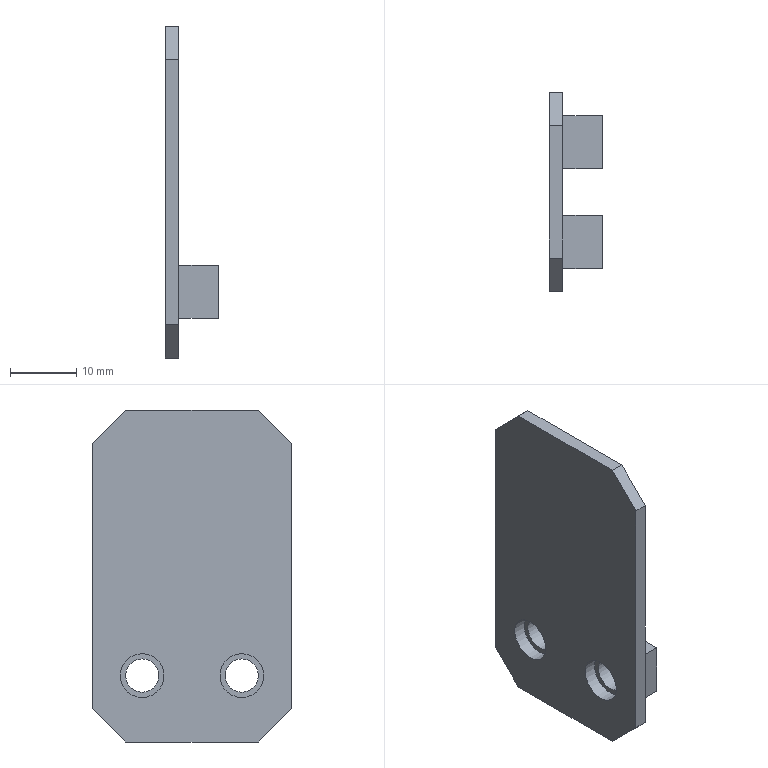Part | NX | features 5003_223_Plate 2 | 1 solid | 26 faces | box 8 x 30 x 50 mm | volume 3296 mm3 | plane 22 | cylinder 4 | commonest cylinder face diameters 5 x2 6.6 x2
STEP:
#1=CARTESIAN_POINT('',(193.825,63.4,-12.));
#2=VERTEX_POINT('',#1);
#3=CARTESIAN_POINT('',(193.825,68.4,-7.));
#4=VERTEX_POINT('',#3);
#5=CARTESIAN_POINT('',(193.825,63.4,-12.));
#6=DIRECTION('',(0.,0.7071,0.7071));
#7=VECTOR('',#6,1000.);
#8=LINE('',#5,#7);
#9=EDGE_CURVE('',#2,#4,#8,.T.);
#10=ORIENTED_EDGE('',*,*,#9,.T.);
#11=CARTESIAN_POINT('',(193.825,88.4,-7.));
#12=VERTEX_POINT('',#11);
#13=CARTESIAN_POINT('',(193.825,88.4,-7.));
#14=DIRECTION('',(0.,1.,0.));
#15=VECTOR('',#14,1000.);
#16=LINE('',#13,#15);
#17=EDGE_CURVE('',#4,#12,#16,.T.);
#18=ORIENTED_EDGE('',*,*,#17,.T.);
#19=CARTESIAN_POINT('',(193.825,93.4,-12.));
#20=VERTEX_POINT('',#19);
#21=CARTESIAN_POINT('',(193.825,93.4,-12.));
#22=DIRECTION('',(0.,0.7071,-0.7071));
#23=VECTOR('',#22,1000.);
#24=LINE('',#21,#23);
#25=EDGE_CURVE('',#12,#20,#24,.T.);
#26=ORIENTED_EDGE('',*,*,#25,.T.);
#27=CARTESIAN_POINT('',(193.825,93.4,-52.));
#28=VERTEX_POINT('',#27);
#29=CARTESIAN_POINT('',(193.825,93.4,-52.));
#30=DIRECTION('',(0.,0.,-1.));
#31=VECTOR('',#30,1000.);
#32=LINE('',#29,#31);
#33=EDGE_CURVE('',#20,#28,#32,.T.);
#34=ORIENTED_EDGE('',*,*,#33,.T.);
#35=CARTESIAN_POINT('',(193.825,88.4,-57.));
#36=VERTEX_POINT('',#35);
#37=CARTESIAN_POINT('',(193.825,88.4,-57.));
#38=DIRECTION('',(0.,-0.7071,-0.7071));
#39=VECTOR('',#38,1000.);
#40=LINE('',#37,#39);
#41=EDGE_CURVE('',#28,#36,#40,.T.);
#42=ORIENTED_EDGE('',*,*,#41,.T.);
#43=CARTESIAN_POINT('',(193.825,68.4,-57.));
#44=VERTEX_POINT('',#43);
#45=CARTESIAN_POINT('',(193.825,88.4,-57.));
#46=DIRECTION('',(0.,-1.,0.));
#47=VECTOR('',#46,1000.);
#48=LINE('',#45,#47);
#49=EDGE_CURVE('',#36,#44,#48,.T.);
#50=ORIENTED_EDGE('',*,*,#49,.T.);
#51=CARTESIAN_POINT('',(193.825,63.4,-52.));
#52=VERTEX_POINT('',#51);
#53=CARTESIAN_POINT('',(193.825,68.4,-57.));
#54=DIRECTION('',(0.,-0.7071,0.7071));
#55=VECTOR('',#54,1000.);
#56=LINE('',#53,#55);
#57=EDGE_CURVE('',#44,#52,#56,.T.);
#58=ORIENTED_EDGE('',*,*,#57,.T.);
#59=CARTESIAN_POINT('',(193.825,63.4,-52.));
#60=DIRECTION('',(0.,0.,1.));
#61=VECTOR('',#60,1000.);
#62=LINE('',#59,#61);
#63=EDGE_CURVE('',#52,#2,#62,.T.);
#64=ORIENTED_EDGE('',*,*,#63,.T.);
#65=EDGE_LOOP('',(#10,#18,#26,#34,#42,#50,#58,#64));
#66=FACE_BOUND('',#65,.T.);
#67=CARTESIAN_POINT('',(193.825,85.9,-50.3));
#68=VERTEX_POINT('',#67);
#69=CARTESIAN_POINT('',(193.825,85.9,-47.));
#70=DIRECTION('',(-1.,0.,0.));
#71=DIRECTION('',(0.,0.,-1.));
#72=AXIS2_PLACEMENT_3D('',#69,#70,#71);
#73=CIRCLE('',#72,3.3);
#74=EDGE_CURVE('',#68,#68,#73,.T.);
#75=ORIENTED_EDGE('',*,*,#74,.F.);
#76=EDGE_LOOP('',(#75));
#77=FACE_BOUND('',#76,.T.);
#78=CARTESIAN_POINT('',(193.825,70.9,-50.3));
#79=VERTEX_POINT('',#78);
#80=CARTESIAN_POINT('',(193.825,70.9,-47.));
#81=DIRECTION('',(-1.,0.,0.));
#82=DIRECTION('',(0.,0.,-1.));
#83=AXIS2_PLACEMENT_3D('',#80,#81,#82);
#84=CIRCLE('',#83,3.3);
#85=EDGE_CURVE('',#79,#79,#84,.T.);
#86=ORIENTED_EDGE('',*,*,#85,.F.);
#87=EDGE_LOOP('',(#86));
#88=FACE_BOUND('',#87,.T.);
#89=CARTESIAN_POINT('',(193.825,93.4,-57.));
#90=DIRECTION('',(1.,0.,0.));
#91=DIRECTION('',(0.,0.,1.));
#92=AXIS2_PLACEMENT_3D('',#89,#90,#91);
#93=PLANE('',#92);
#94=ADVANCED_FACE('',(#66,#77,#88),#93,.F.);
#95=CARTESIAN_POINT('',(195.825,89.9,-51.));
#96=VERTEX_POINT('',#95);
#97=CARTESIAN_POINT('',(195.825,81.9,-51.));
#98=VERTEX_POINT('',#97);
#99=CARTESIAN_POINT('',(195.825,81.9,-51.));
#100=DIRECTION('',(0.,-1.,0.));
#101=VECTOR('',#100,1000.);
#102=LINE('',#99,#101);
#103=EDGE_CURVE('',#96,#98,#102,.T.);
#104=ORIENTED_EDGE('',*,*,#103,.T.);
#105=CARTESIAN_POINT('',(195.825,81.9,-43.));
#106=VERTEX_POINT('',#105);
#107=CARTESIAN_POINT('',(195.825,81.9,-43.));
#108=DIRECTION('',(0.,0.,1.));
#109=VECTOR('',#108,1000.);
#110=LINE('',#107,#109);
#111=EDGE_CURVE('',#98,#106,#110,.T.);
#112=ORIENTED_EDGE('',*,*,#111,.T.);
#113=CARTESIAN_POINT('',(195.825,89.9,-43.));
#114=VERTEX_POINT('',#113);
#115=CARTESIAN_POINT('',(195.825,81.9,-43.));
#116=DIRECTION('',(0.,1.,0.));
#117=VECTOR('',#116,1000.);
#118=LINE('',#115,#117);
#119=EDGE_CURVE('',#106,#114,#118,.T.);
#120=ORIENTED_EDGE('',*,*,#119,.T.);
#121=CARTESIAN_POINT('',(195.825,89.9,-43.));
#122=DIRECTION('',(0.,0.,-1.));
#123=VECTOR('',#122,1000.);
#124=LINE('',#121,#123);
#125=EDGE_CURVE('',#114,#96,#124,.T.);
#126=ORIENTED_EDGE('',*,*,#125,.T.);
#127=EDGE_LOOP('',(#104,#112,#120,#126));
#128=FACE_BOUND('',#127,.T.);
#129=CARTESIAN_POINT('',(195.825,74.9,-51.));
#130=VERTEX_POINT('',#129);
#131=CARTESIAN_POINT('',(195.825,66.9,-51.));
#132=VERTEX_POINT('',#131);
#133=CARTESIAN_POINT('',(195.825,66.9,-51.));
#134=DIRECTION('',(0.,-1.,0.));
#135=VECTOR('',#134,1000.);
#136=LINE('',#133,#135);
#137=EDGE_CURVE('',#130,#132,#136,.T.);
#138=ORIENTED_EDGE('',*,*,#137,.T.);
#139=CARTESIAN_POINT('',(195.825,66.9,-43.));
#140=VERTEX_POINT('',#139);
#141=CARTESIAN_POINT('',(195.825,66.9,-43.));
#142=DIRECTION('',(0.,0.,1.));
#143=VECTOR('',#142,1000.);
#144=LINE('',#141,#143);
#145=EDGE_CURVE('',#132,#140,#144,.T.);
#146=ORIENTED_EDGE('',*,*,#145,.T.);
#147=CARTESIAN_POINT('',(195.825,74.9,-43.));
#148=VERTEX_POINT('',#147);
#149=CARTESIAN_POINT('',(195.825,66.9,-43.));
#150=DIRECTION('',(0.,1.,0.));
#151=VECTOR('',#150,1000.);
#152=LINE('',#149,#151);
#153=EDGE_CURVE('',#140,#148,#152,.T.);
#154=ORIENTED_EDGE('',*,*,#153,.T.);
#155=CARTESIAN_POINT('',(195.825,74.9,-43.));
#156=DIRECTION('',(0.,0.,-1.));
#157=VECTOR('',#156,1000.);
#158=LINE('',#155,#157);
#159=EDGE_CURVE('',#148,#130,#158,.T.);
#160=ORIENTED_EDGE('',*,*,#159,.T.);
#161=EDGE_LOOP('',(#138,#146,#154,#160));
#162=FACE_BOUND('',#161,.T.);
#163=CARTESIAN_POINT('',(195.825,63.4,-12.));
#164=VERTEX_POINT('',#163);
#165=CARTESIAN_POINT('',(195.825,68.4,-7.));
#166=VERTEX_POINT('',#165);
#167=CARTESIAN_POINT('',(195.825,63.4,-12.));
#168=DIRECTION('',(0.,0.7071,0.7071));
#169=VECTOR('',#168,1000.);
#170=LINE('',#167,#169);
#171=EDGE_CURVE('',#164,#166,#170,.T.);
#172=ORIENTED_EDGE('',*,*,#171,.F.);
#173=CARTESIAN_POINT('',(195.825,63.4,-52.));
#174=VERTEX_POINT('',#173);
#175=CARTESIAN_POINT('',(195.825,63.4,-52.));
#176=DIRECTION('',(0.,0.,1.));
#177=VECTOR('',#176,1000.);
#178=LINE('',#175,#177);
#179=EDGE_CURVE('',#174,#164,#178,.T.);
#180=ORIENTED_EDGE('',*,*,#179,.F.);
#181=CARTESIAN_POINT('',(195.825,68.4,-57.));
#182=VERTEX_POINT('',#181);
#183=CARTESIAN_POINT('',(195.825,68.4,-57.));
#184=DIRECTION('',(0.,-0.7071,0.7071));
#185=VECTOR('',#184,1000.);
#186=LINE('',#183,#185);
#187=EDGE_CURVE('',#182,#174,#186,.T.);
#188=ORIENTED_EDGE('',*,*,#187,.F.);
#189=CARTESIAN_POINT('',(195.825,88.4,-57.));
#190=VERTEX_POINT('',#189);
#191=CARTESIAN_POINT('',(195.825,88.4,-57.));
#192=DIRECTION('',(0.,-1.,0.));
#193=VECTOR('',#192,1000.);
#194=LINE('',#191,#193);
#195=EDGE_CURVE('',#190,#182,#194,.T.);
#196=ORIENTED_EDGE('',*,*,#195,.F.);
#197=CARTESIAN_POINT('',(195.825,93.4,-52.));
#198=VERTEX_POINT('',#197);
#199=CARTESIAN_POINT('',(195.825,88.4,-57.));
#200=DIRECTION('',(0.,-0.7071,-0.7071));
#201=VECTOR('',#200,1000.);
#202=LINE('',#199,#201);
#203=EDGE_CURVE('',#198,#190,#202,.T.);
#204=ORIENTED_EDGE('',*,*,#203,.F.);
#205=CARTESIAN_POINT('',(195.825,93.4,-12.));
#206=VERTEX_POINT('',#205);
#207=CARTESIAN_POINT('',(195.825,93.4,-52.));
#208=DIRECTION('',(0.,0.,-1.));
#209=VECTOR('',#208,1000.);
#210=LINE('',#207,#209);
#211=EDGE_CURVE('',#206,#198,#210,.T.);
#212=ORIENTED_EDGE('',*,*,#211,.F.);
#213=CARTESIAN_POINT('',(195.825,88.4,-7.));
#214=VERTEX_POINT('',#213);
#215=CARTESIAN_POINT('',(195.825,93.4,-12.));
#216=DIRECTION('',(0.,0.7071,-0.7071));
#217=VECTOR('',#216,1000.);
#218=LINE('',#215,#217);
#219=EDGE_CURVE('',#214,#206,#218,.T.);
#220=ORIENTED_EDGE('',*,*,#219,.F.);
#221=CARTESIAN_POINT('',(195.825,88.4,-7.));
#222=DIRECTION('',(0.,1.,0.));
#223=VECTOR('',#222,1000.);
#224=LINE('',#221,#223);
#225=EDGE_CURVE('',#166,#214,#224,.T.);
#226=ORIENTED_EDGE('',*,*,#225,.F.);
#227=EDGE_LOOP('',(#172,#180,#188,#196,#204,#212,#220,#226));
#228=FACE_BOUND('',#227,.T.);
#229=CARTESIAN_POINT('',(195.825,93.4,-57.));
#230=DIRECTION('',(1.,0.,0.));
#231=DIRECTION('',(0.,0.,1.));
#232=AXIS2_PLACEMENT_3D('',#229,#230,#231);
#233=PLANE('',#232);
#234=ADVANCED_FACE('',(#128,#162,#228),#233,.T.);
#235=ORIENTED_EDGE('',*,*,#171,.T.);
#236=CARTESIAN_POINT('',(193.825,68.4,-7.));
#237=DIRECTION('',(1.,0.,0.));
#238=VECTOR('',#237,1000.);
#239=LINE('',#236,#238);
#240=EDGE_CURVE('',#4,#166,#239,.T.);
#241=ORIENTED_EDGE('',*,*,#240,.F.);
#242=ORIENTED_EDGE('',*,*,#9,.F.);
#243=CARTESIAN_POINT('',(193.825,63.4,-12.));
#244=DIRECTION('',(1.,0.,0.));
#245=VECTOR('',#244,1000.);
#246=LINE('',#243,#245);
#247=EDGE_CURVE('',#2,#164,#246,.T.);
#248=ORIENTED_EDGE('',*,*,#247,.T.);
#249=EDGE_LOOP('',(#235,#241,#242,#248));
#250=FACE_BOUND('',#249,.T.);
#251=CARTESIAN_POINT('',(193.825,63.4,-12.));
#252=DIRECTION('',(0.,0.7071,-0.7071));
#253=DIRECTION('',(0.,-0.7071,-0.7071));
#254=AXIS2_PLACEMENT_3D('',#251,#252,#253);
#255=PLANE('',#254);
#256=ADVANCED_FACE('',(#250),#255,.F.);
#257=ORIENTED_EDGE('',*,*,#225,.T.);
#258=CARTESIAN_POINT('',(193.825,88.4,-7.));
#259=DIRECTION('',(1.,0.,0.));
#260=VECTOR('',#259,1000.);
#261=LINE('',#258,#260);
#262=EDGE_CURVE('',#12,#214,#261,.T.);
#263=ORIENTED_EDGE('',*,*,#262,.F.);
#264=ORIENTED_EDGE('',*,*,#17,.F.);
#265=ORIENTED_EDGE('',*,*,#240,.T.);
#266=EDGE_LOOP('',(#257,#263,#264,#265));
#267=FACE_BOUND('',#266,.T.);
#268=CARTESIAN_POINT('',(193.825,88.4,-7.));
#269=DIRECTION('',(0.,0.,-1.));
#270=DIRECTION('',(1.,0.,0.));
#271=AXIS2_PLACEMENT_3D('',#268,#269,#270);
#272=PLANE('',#271);
#273=ADVANCED_FACE('',(#267),#272,.F.);
#274=ORIENTED_EDGE('',*,*,#219,.T.);
#275=CARTESIAN_POINT('',(193.825,93.4,-12.));
#276=DIRECTION('',(1.,0.,0.));
#277=VECTOR('',#276,1000.);
#278=LINE('',#275,#277);
#279=EDGE_CURVE('',#20,#206,#278,.T.);
#280=ORIENTED_EDGE('',*,*,#279,.F.);
#281=ORIENTED_EDGE('',*,*,#25,.F.);
#282=ORIENTED_EDGE('',*,*,#262,.T.);
#283=EDGE_LOOP('',(#274,#280,#281,#282));
#284=FACE_BOUND('',#283,.T.);
#285=CARTESIAN_POINT('',(193.825,93.4,-12.));
#286=DIRECTION('',(0.,-0.7071,-0.7071));
#287=DIRECTION('',(0.,-0.7071,0.7071));
#288=AXIS2_PLACEMENT_3D('',#285,#286,#287);
#289=PLANE('',#288);
#290=ADVANCED_FACE('',(#284),#289,.F.);
#291=ORIENTED_EDGE('',*,*,#211,.T.);
#292=CARTESIAN_POINT('',(193.825,93.4,-52.));
#293=DIRECTION('',(1.,0.,0.));
#294=VECTOR('',#293,1000.);
#295=LINE('',#292,#294);
#296=EDGE_CURVE('',#28,#198,#295,.T.);
#297=ORIENTED_EDGE('',*,*,#296,.F.);
#298=ORIENTED_EDGE('',*,*,#33,.F.);
#299=ORIENTED_EDGE('',*,*,#279,.T.);
#300=EDGE_LOOP('',(#291,#297,#298,#299));
#301=FACE_BOUND('',#300,.T.);
#302=CARTESIAN_POINT('',(193.825,93.4,-52.));
#303=DIRECTION('',(0.,-1.,0.));
#304=DIRECTION('',(0.,0.,1.));
#305=AXIS2_PLACEMENT_3D('',#302,#303,#304);
#306=PLANE('',#305);
#307=ADVANCED_FACE('',(#301),#306,.F.);
#308=ORIENTED_EDGE('',*,*,#203,.T.);
#309=CARTESIAN_POINT('',(193.825,88.4,-57.));
#310=DIRECTION('',(1.,0.,0.));
#311=VECTOR('',#310,1000.);
#312=LINE('',#309,#311);
#313=EDGE_CURVE('',#36,#190,#312,.T.);
#314=ORIENTED_EDGE('',*,*,#313,.F.);
#315=ORIENTED_EDGE('',*,*,#41,.F.);
#316=ORIENTED_EDGE('',*,*,#296,.T.);
#317=EDGE_LOOP('',(#308,#314,#315,#316));
#318=FACE_BOUND('',#317,.T.);
#319=CARTESIAN_POINT('',(193.825,88.4,-57.));
#320=DIRECTION('',(0.,-0.7071,0.7071));
#321=DIRECTION('',(0.,0.7071,0.7071));
#322=AXIS2_PLACEMENT_3D('',#319,#320,#321);
#323=PLANE('',#322);
#324=ADVANCED_FACE('',(#318),#323,.F.);
#325=ORIENTED_EDGE('',*,*,#195,.T.);
#326=CARTESIAN_POINT('',(193.825,68.4,-57.));
#327=DIRECTION('',(1.,0.,0.));
#328=VECTOR('',#327,1000.);
#329=LINE('',#326,#328);
#330=EDGE_CURVE('',#44,#182,#329,.T.);
#331=ORIENTED_EDGE('',*,*,#330,.F.);
#332=ORIENTED_EDGE('',*,*,#49,.F.);
#333=ORIENTED_EDGE('',*,*,#313,.T.);
#334=EDGE_LOOP('',(#325,#331,#332,#333));
#335=FACE_BOUND('',#334,.T.);
#336=CARTESIAN_POINT('',(193.825,88.4,-57.));
#337=DIRECTION('',(0.,0.,1.));
#338=DIRECTION('',(-1.,0.,0.));
#339=AXIS2_PLACEMENT_3D('',#336,#337,#338);
#340=PLANE('',#339);
#341=ADVANCED_FACE('',(#335),#340,.F.);
#342=ORIENTED_EDGE('',*,*,#187,.T.);
#343=CARTESIAN_POINT('',(193.825,63.4,-52.));
#344=DIRECTION('',(1.,0.,0.));
#345=VECTOR('',#344,1000.);
#346=LINE('',#343,#345);
#347=EDGE_CURVE('',#52,#174,#346,.T.);
#348=ORIENTED_EDGE('',*,*,#347,.F.);
#349=ORIENTED_EDGE('',*,*,#57,.F.);
#350=ORIENTED_EDGE('',*,*,#330,.T.);
#351=EDGE_LOOP('',(#342,#348,#349,#350));
#352=FACE_BOUND('',#351,.T.);
#353=CARTESIAN_POINT('',(193.825,68.4,-57.));
#354=DIRECTION('',(0.,0.7071,0.7071));
#355=DIRECTION('',(0.,0.7071,-0.7071));
#356=AXIS2_PLACEMENT_3D('',#353,#354,#355);
#357=PLANE('',#356);
#358=ADVANCED_FACE('',(#352),#357,.F.);
#359=ORIENTED_EDGE('',*,*,#179,.T.);
#360=ORIENTED_EDGE('',*,*,#247,.F.);
#361=ORIENTED_EDGE('',*,*,#63,.F.);
#362=ORIENTED_EDGE('',*,*,#347,.T.);
#363=EDGE_LOOP('',(#359,#360,#361,#362));
#364=FACE_BOUND('',#363,.T.);
#365=CARTESIAN_POINT('',(193.825,63.4,-52.));
#366=DIRECTION('',(0.,1.,0.));
#367=DIRECTION('',(0.,0.,-1.));
#368=AXIS2_PLACEMENT_3D('',#365,#366,#367);
#369=PLANE('',#368);
#370=ADVANCED_FACE('',(#364),#369,.F.);
#371=ORIENTED_EDGE('',*,*,#74,.T.);
#372=EDGE_LOOP('',(#371));
#373=FACE_BOUND('',#372,.T.);
#374=CARTESIAN_POINT('',(195.825,85.9,-50.3));
#375=VERTEX_POINT('',#374);
#376=CARTESIAN_POINT('',(195.825,85.9,-47.));
#377=DIRECTION('',(-1.,0.,0.));
#378=DIRECTION('',(0.,0.,-1.));
#379=AXIS2_PLACEMENT_3D('',#376,#377,#378);
#380=CIRCLE('',#379,3.3);
#381=EDGE_CURVE('',#375,#375,#380,.T.);
#382=ORIENTED_EDGE('',*,*,#381,.F.);
#383=EDGE_LOOP('',(#382));
#384=FACE_BOUND('',#383,.T.);
#385=CARTESIAN_POINT('',(193.825,85.9,-47.));
#386=DIRECTION('',(1.,0.,0.));
#387=DIRECTION('',(0.,0.,1.));
#388=AXIS2_PLACEMENT_3D('',#385,#386,#387);
#389=CYLINDRICAL_SURFACE('',#388,3.3);
#390=ADVANCED_FACE('',(#373,#384),#389,.F.);
#391=ORIENTED_EDGE('',*,*,#85,.T.);
#392=EDGE_LOOP('',(#391));
#393=FACE_BOUND('',#392,.T.);
#394=CARTESIAN_POINT('',(195.825,70.9,-50.3));
#395=VERTEX_POINT('',#394);
#396=CARTESIAN_POINT('',(195.825,70.9,-47.));
#397=DIRECTION('',(-1.,0.,0.));
#398=DIRECTION('',(0.,0.,-1.));
#399=AXIS2_PLACEMENT_3D('',#396,#397,#398);
#400=CIRCLE('',#399,3.3);
#401=EDGE_CURVE('',#395,#395,#400,.T.);
#402=ORIENTED_EDGE('',*,*,#401,.F.);
#403=EDGE_LOOP('',(#402));
#404=FACE_BOUND('',#403,.T.);
#405=CARTESIAN_POINT('',(193.825,70.9,-47.));
#406=DIRECTION('',(1.,0.,0.));
#407=DIRECTION('',(0.,0.,1.));
#408=AXIS2_PLACEMENT_3D('',#405,#406,#407);
#409=CYLINDRICAL_SURFACE('',#408,3.3);
#410=ADVANCED_FACE('',(#393,#404),#409,.F.);
#411=CARTESIAN_POINT('',(195.825,70.9,-49.5));
#412=VERTEX_POINT('',#411);
#413=CARTESIAN_POINT('',(195.825,70.9,-47.));
#414=DIRECTION('',(-1.,0.,0.));
#415=DIRECTION('',(0.,0.,-1.));
#416=AXIS2_PLACEMENT_3D('',#413,#414,#415);
#417=CIRCLE('',#416,2.5);
#418=EDGE_CURVE('',#412,#412,#417,.T.);
#419=ORIENTED_EDGE('',*,*,#418,.F.);
#420=EDGE_LOOP('',(#419));
#421=FACE_BOUND('',#420,.T.);
#422=ORIENTED_EDGE('',*,*,#401,.T.);
#423=EDGE_LOOP('',(#422));
#424=FACE_BOUND('',#423,.T.);
#425=CARTESIAN_POINT('',(195.825,93.4,-57.));
#426=DIRECTION('',(-1.,0.,0.));
#427=DIRECTION('',(0.,0.,-1.));
#428=AXIS2_PLACEMENT_3D('',#425,#426,#427);
#429=PLANE('',#428);
#430=ADVANCED_FACE('',(#421,#424),#429,.T.);
#431=ORIENTED_EDGE('',*,*,#137,.F.);
#432=CARTESIAN_POINT('',(201.825,74.9,-51.));
#433=VERTEX_POINT('',#432);
#434=CARTESIAN_POINT('',(201.825,74.9,-51.));
#435=DIRECTION('',(-1.,0.,0.));
#436=VECTOR('',#435,1000.);
#437=LINE('',#434,#436);
#438=EDGE_CURVE('',#433,#130,#437,.T.);
#439=ORIENTED_EDGE('',*,*,#438,.F.);
#440=CARTESIAN_POINT('',(201.825,66.9,-51.));
#441=VERTEX_POINT('',#440);
#442=CARTESIAN_POINT('',(201.825,66.9,-51.));
#443=DIRECTION('',(0.,-1.,0.));
#444=VECTOR('',#443,1000.);
#445=LINE('',#442,#444);
#446=EDGE_CURVE('',#433,#441,#445,.T.);
#447=ORIENTED_EDGE('',*,*,#446,.T.);
#448=CARTESIAN_POINT('',(201.825,66.9,-51.));
#449=DIRECTION('',(-1.,0.,0.));
#450=VECTOR('',#449,1000.);
#451=LINE('',#448,#450);
#452=EDGE_CURVE('',#441,#132,#451,.T.);
#453=ORIENTED_EDGE('',*,*,#452,.T.);
#454=EDGE_LOOP('',(#431,#439,#447,#453));
#455=FACE_BOUND('',#454,.T.);
#456=CARTESIAN_POINT('',(201.825,66.9,-51.));
#457=DIRECTION('',(0.,0.,-1.));
#458=DIRECTION('',(0.,-1.,0.));
#459=AXIS2_PLACEMENT_3D('',#456,#457,#458);
#460=PLANE('',#459);
#461=ADVANCED_FACE('',(#455),#460,.T.);
#462=ORIENTED_EDGE('',*,*,#159,.F.);
#463=CARTESIAN_POINT('',(201.825,74.9,-43.));
#464=VERTEX_POINT('',#463);
#465=CARTESIAN_POINT('',(201.825,74.9,-43.));
#466=DIRECTION('',(-1.,0.,0.));
#467=VECTOR('',#466,1000.);
#468=LINE('',#465,#467);
#469=EDGE_CURVE('',#464,#148,#468,.T.);
#470=ORIENTED_EDGE('',*,*,#469,.F.);
#471=CARTESIAN_POINT('',(201.825,74.9,-43.));
#472=DIRECTION('',(0.,0.,-1.));
#473=VECTOR('',#472,1000.);
#474=LINE('',#471,#473);
#475=EDGE_CURVE('',#464,#433,#474,.T.);
#476=ORIENTED_EDGE('',*,*,#475,.T.);
#477=ORIENTED_EDGE('',*,*,#438,.T.);
#478=EDGE_LOOP('',(#462,#470,#476,#477));
#479=FACE_BOUND('',#478,.T.);
#480=CARTESIAN_POINT('',(201.825,74.9,-43.));
#481=DIRECTION('',(0.,1.,0.));
#482=DIRECTION('',(0.,0.,-1.));
#483=AXIS2_PLACEMENT_3D('',#480,#481,#482);
#484=PLANE('',#483);
#485=ADVANCED_FACE('',(#479),#484,.T.);
#486=ORIENTED_EDGE('',*,*,#153,.F.);
#487=CARTESIAN_POINT('',(201.825,66.9,-43.));
#488=VERTEX_POINT('',#487);
#489=CARTESIAN_POINT('',(201.825,66.9,-43.));
#490=DIRECTION('',(-1.,0.,0.));
#491=VECTOR('',#490,1000.);
#492=LINE('',#489,#491);
#493=EDGE_CURVE('',#488,#140,#492,.T.);
#494=ORIENTED_EDGE('',*,*,#493,.F.);
#495=CARTESIAN_POINT('',(201.825,66.9,-43.));
#496=DIRECTION('',(0.,1.,0.));
#497=VECTOR('',#496,1000.);
#498=LINE('',#495,#497);
#499=EDGE_CURVE('',#488,#464,#498,.T.);
#500=ORIENTED_EDGE('',*,*,#499,.T.);
#501=ORIENTED_EDGE('',*,*,#469,.T.);
#502=EDGE_LOOP('',(#486,#494,#500,#501));
#503=FACE_BOUND('',#502,.T.);
#504=CARTESIAN_POINT('',(201.825,66.9,-43.));
#505=DIRECTION('',(0.,0.,1.));
#506=DIRECTION('',(0.,1.,0.));
#507=AXIS2_PLACEMENT_3D('',#504,#505,#506);
#508=PLANE('',#507);
#509=ADVANCED_FACE('',(#503),#508,.T.);
#510=ORIENTED_EDGE('',*,*,#145,.F.);
#511=ORIENTED_EDGE('',*,*,#452,.F.);
#512=CARTESIAN_POINT('',(201.825,66.9,-43.));
#513=DIRECTION('',(0.,0.,1.));
#514=VECTOR('',#513,1000.);
#515=LINE('',#512,#514);
#516=EDGE_CURVE('',#441,#488,#515,.T.);
#517=ORIENTED_EDGE('',*,*,#516,.T.);
#518=ORIENTED_EDGE('',*,*,#493,.T.);
#519=EDGE_LOOP('',(#510,#511,#517,#518));
#520=FACE_BOUND('',#519,.T.);
#521=CARTESIAN_POINT('',(201.825,66.9,-43.));
#522=DIRECTION('',(0.,-1.,0.));
#523=DIRECTION('',(0.,0.,1.));
#524=AXIS2_PLACEMENT_3D('',#521,#522,#523);
#525=PLANE('',#524);
#526=ADVANCED_FACE('',(#520),#525,.T.);
#527=CARTESIAN_POINT('',(201.825,70.9,-49.5));
#528=VERTEX_POINT('',#527);
#529=CARTESIAN_POINT('',(201.825,70.9,-47.));
#530=DIRECTION('',(-1.,0.,0.));
#531=DIRECTION('',(0.,0.,-1.));
#532=AXIS2_PLACEMENT_3D('',#529,#530,#531);
#533=CIRCLE('',#532,2.5);
#534=EDGE_CURVE('',#528,#528,#533,.T.);
#535=ORIENTED_EDGE('',*,*,#534,.T.);
#536=EDGE_LOOP('',(#535));
#537=FACE_BOUND('',#536,.T.);
#538=ORIENTED_EDGE('',*,*,#446,.F.);
#539=ORIENTED_EDGE('',*,*,#475,.F.);
#540=ORIENTED_EDGE('',*,*,#499,.F.);
#541=ORIENTED_EDGE('',*,*,#516,.F.);
#542=EDGE_LOOP('',(#538,#539,#540,#541));
#543=FACE_BOUND('',#542,.T.);
#544=CARTESIAN_POINT('',(201.825,93.4,-57.));
#545=DIRECTION('',(-1.,0.,0.));
#546=DIRECTION('',(0.,0.,-1.));
#547=AXIS2_PLACEMENT_3D('',#544,#545,#546);
#548=PLANE('',#547);
#549=ADVANCED_FACE('',(#537,#543),#548,.F.);
#550=CARTESIAN_POINT('',(195.825,85.9,-49.5));
#551=VERTEX_POINT('',#550);
#552=CARTESIAN_POINT('',(195.825,85.9,-47.));
#553=DIRECTION('',(-1.,0.,0.));
#554=DIRECTION('',(0.,0.,-1.));
#555=AXIS2_PLACEMENT_3D('',#552,#553,#554);
#556=CIRCLE('',#555,2.5);
#557=EDGE_CURVE('',#551,#551,#556,.T.);
#558=ORIENTED_EDGE('',*,*,#557,.F.);
#559=EDGE_LOOP('',(#558));
#560=FACE_BOUND('',#559,.T.);
#561=ORIENTED_EDGE('',*,*,#381,.T.);
#562=EDGE_LOOP('',(#561));
#563=FACE_BOUND('',#562,.T.);
#564=CARTESIAN_POINT('',(195.825,93.4,-57.));
#565=DIRECTION('',(-1.,0.,0.));
#566=DIRECTION('',(0.,0.,-1.));
#567=AXIS2_PLACEMENT_3D('',#564,#565,#566);
#568=PLANE('',#567);
#569=ADVANCED_FACE('',(#560,#563),#568,.T.);
#570=ORIENTED_EDGE('',*,*,#103,.F.);
#571=CARTESIAN_POINT('',(201.825,89.9,-51.));
#572=VERTEX_POINT('',#571);
#573=CARTESIAN_POINT('',(201.825,89.9,-51.));
#574=DIRECTION('',(-1.,0.,0.));
#575=VECTOR('',#574,1000.);
#576=LINE('',#573,#575);
#577=EDGE_CURVE('',#572,#96,#576,.T.);
#578=ORIENTED_EDGE('',*,*,#577,.F.);
#579=CARTESIAN_POINT('',(201.825,81.9,-51.));
#580=VERTEX_POINT('',#579);
#581=CARTESIAN_POINT('',(201.825,81.9,-51.));
#582=DIRECTION('',(0.,-1.,0.));
#583=VECTOR('',#582,1000.);
#584=LINE('',#581,#583);
#585=EDGE_CURVE('',#572,#580,#584,.T.);
#586=ORIENTED_EDGE('',*,*,#585,.T.);
#587=CARTESIAN_POINT('',(201.825,81.9,-51.));
#588=DIRECTION('',(-1.,0.,0.));
#589=VECTOR('',#588,1000.);
#590=LINE('',#587,#589);
#591=EDGE_CURVE('',#580,#98,#590,.T.);
#592=ORIENTED_EDGE('',*,*,#591,.T.);
#593=EDGE_LOOP('',(#570,#578,#586,#592));
#594=FACE_BOUND('',#593,.T.);
#595=CARTESIAN_POINT('',(201.825,81.9,-51.));
#596=DIRECTION('',(0.,0.,-1.));
#597=DIRECTION('',(1.,0.,0.));
#598=AXIS2_PLACEMENT_3D('',#595,#596,#597);
#599=PLANE('',#598);
#600=ADVANCED_FACE('',(#594),#599,.T.);
#601=ORIENTED_EDGE('',*,*,#125,.F.);
#602=CARTESIAN_POINT('',(201.825,89.9,-43.));
#603=VERTEX_POINT('',#602);
#604=CARTESIAN_POINT('',(201.825,89.9,-43.));
#605=DIRECTION('',(-1.,0.,0.));
#606=VECTOR('',#605,1000.);
#607=LINE('',#604,#606);
#608=EDGE_CURVE('',#603,#114,#607,.T.);
#609=ORIENTED_EDGE('',*,*,#608,.F.);
#610=CARTESIAN_POINT('',(201.825,89.9,-43.));
#611=DIRECTION('',(0.,0.,-1.));
#612=VECTOR('',#611,1000.);
#613=LINE('',#610,#612);
#614=EDGE_CURVE('',#603,#572,#613,.T.);
#615=ORIENTED_EDGE('',*,*,#614,.T.);
#616=ORIENTED_EDGE('',*,*,#577,.T.);
#617=EDGE_LOOP('',(#601,#609,#615,#616));
#618=FACE_BOUND('',#617,.T.);
#619=CARTESIAN_POINT('',(201.825,89.9,-43.));
#620=DIRECTION('',(0.,1.,0.));
#621=DIRECTION('',(0.,0.,-1.));
#622=AXIS2_PLACEMENT_3D('',#619,#620,#621);
#623=PLANE('',#622);
#624=ADVANCED_FACE('',(#618),#623,.T.);
#625=ORIENTED_EDGE('',*,*,#119,.F.);
#626=CARTESIAN_POINT('',(201.825,81.9,-43.));
#627=VERTEX_POINT('',#626);
#628=CARTESIAN_POINT('',(201.825,81.9,-43.));
#629=DIRECTION('',(-1.,0.,0.));
#630=VECTOR('',#629,1000.);
#631=LINE('',#628,#630);
#632=EDGE_CURVE('',#627,#106,#631,.T.);
#633=ORIENTED_EDGE('',*,*,#632,.F.);
#634=CARTESIAN_POINT('',(201.825,81.9,-43.));
#635=DIRECTION('',(0.,1.,0.));
#636=VECTOR('',#635,1000.);
#637=LINE('',#634,#636);
#638=EDGE_CURVE('',#627,#603,#637,.T.);
#639=ORIENTED_EDGE('',*,*,#638,.T.);
#640=ORIENTED_EDGE('',*,*,#608,.T.);
#641=EDGE_LOOP('',(#625,#633,#639,#640));
#642=FACE_BOUND('',#641,.T.);
#643=CARTESIAN_POINT('',(201.825,81.9,-43.));
#644=DIRECTION('',(0.,0.,1.));
#645=DIRECTION('',(0.,1.,0.));
#646=AXIS2_PLACEMENT_3D('',#643,#644,#645);
#647=PLANE('',#646);
#648=ADVANCED_FACE('',(#642),#647,.T.);
#649=ORIENTED_EDGE('',*,*,#111,.F.);
#650=ORIENTED_EDGE('',*,*,#591,.F.);
#651=CARTESIAN_POINT('',(201.825,81.9,-43.));
#652=DIRECTION('',(0.,0.,1.));
#653=VECTOR('',#652,1000.);
#654=LINE('',#651,#653);
#655=EDGE_CURVE('',#580,#627,#654,.T.);
#656=ORIENTED_EDGE('',*,*,#655,.T.);
#657=ORIENTED_EDGE('',*,*,#632,.T.);
#658=EDGE_LOOP('',(#649,#650,#656,#657));
#659=FACE_BOUND('',#658,.T.);
#660=CARTESIAN_POINT('',(201.825,81.9,-43.));
#661=DIRECTION('',(0.,-1.,0.));
#662=DIRECTION('',(0.,0.,1.));
#663=AXIS2_PLACEMENT_3D('',#660,#661,#662);
#664=PLANE('',#663);
#665=ADVANCED_FACE('',(#659),#664,.T.);
#666=CARTESIAN_POINT('',(201.825,85.9,-49.5));
#667=VERTEX_POINT('',#666);
#668=CARTESIAN_POINT('',(201.825,85.9,-47.));
#669=DIRECTION('',(-1.,0.,0.));
#670=DIRECTION('',(0.,0.,-1.));
#671=AXIS2_PLACEMENT_3D('',#668,#669,#670);
#672=CIRCLE('',#671,2.5);
#673=EDGE_CURVE('',#667,#667,#672,.T.);
#674=ORIENTED_EDGE('',*,*,#673,.T.);
#675=EDGE_LOOP('',(#674));
#676=FACE_BOUND('',#675,.T.);
#677=ORIENTED_EDGE('',*,*,#585,.F.);
#678=ORIENTED_EDGE('',*,*,#614,.F.);
#679=ORIENTED_EDGE('',*,*,#638,.F.);
#680=ORIENTED_EDGE('',*,*,#655,.F.);
#681=EDGE_LOOP('',(#677,#678,#679,#680));
#682=FACE_BOUND('',#681,.T.);
#683=CARTESIAN_POINT('',(201.825,93.4,-57.));
#684=DIRECTION('',(-1.,0.,0.));
#685=DIRECTION('',(0.,0.,-1.));
#686=AXIS2_PLACEMENT_3D('',#683,#684,#685);
#687=PLANE('',#686);
#688=ADVANCED_FACE('',(#676,#682),#687,.F.);
#689=ORIENTED_EDGE('',*,*,#534,.F.);
#690=EDGE_LOOP('',(#689));
#691=FACE_BOUND('',#690,.T.);
#692=ORIENTED_EDGE('',*,*,#418,.T.);
#693=EDGE_LOOP('',(#692));
#694=FACE_BOUND('',#693,.T.);
#695=CARTESIAN_POINT('',(195.825,70.9,-47.));
#696=DIRECTION('',(-1.,0.,0.));
#697=DIRECTION('',(0.,0.,-1.));
#698=AXIS2_PLACEMENT_3D('',#695,#696,#697);
#699=CYLINDRICAL_SURFACE('',#698,2.5);
#700=ADVANCED_FACE('',(#691,#694),#699,.F.);
#701=ORIENTED_EDGE('',*,*,#673,.F.);
#702=EDGE_LOOP('',(#701));
#703=FACE_BOUND('',#702,.T.);
#704=ORIENTED_EDGE('',*,*,#557,.T.);
#705=EDGE_LOOP('',(#704));
#706=FACE_BOUND('',#705,.T.);
#707=CARTESIAN_POINT('',(195.825,85.9,-47.));
#708=DIRECTION('',(-1.,0.,0.));
#709=DIRECTION('',(0.,0.,-1.));
#710=AXIS2_PLACEMENT_3D('',#707,#708,#709);
#711=CYLINDRICAL_SURFACE('',#710,2.5);
#712=ADVANCED_FACE('',(#703,#706),#711,.F.);
#713=CLOSED_SHELL('',(#94,#234,#256,#273,#290,#307,#324,#341,#358,#370,#390,#410,#430,#461,#485,#509,#526,#549,#569,#600,#624,#648,#665,#688,#700,#712));
#714=MANIFOLD_SOLID_BREP('',#713);
#715=(LENGTH_UNIT()NAMED_UNIT(*)SI_UNIT(.MILLI.,.METRE.));
#716=UNCERTAINTY_MEASURE_WITH_UNIT(LENGTH_MEASURE(0.00001),#715,'','');
#717=(NAMED_UNIT(*)PLANE_ANGLE_UNIT()SI_UNIT($,.RADIAN.));
#718=(NAMED_UNIT(*)SI_UNIT($,.STERADIAN.)SOLID_ANGLE_UNIT());
#719=(GEOMETRIC_REPRESENTATION_CONTEXT(3)GLOBAL_UNCERTAINTY_ASSIGNED_CONTEXT((#716))GLOBAL_UNIT_ASSIGNED_CONTEXT((#715,#717,#718))REPRESENTATION_CONTEXT('',''));
#720=ADVANCED_BREP_SHAPE_REPRESENTATION('',(#714),#719);